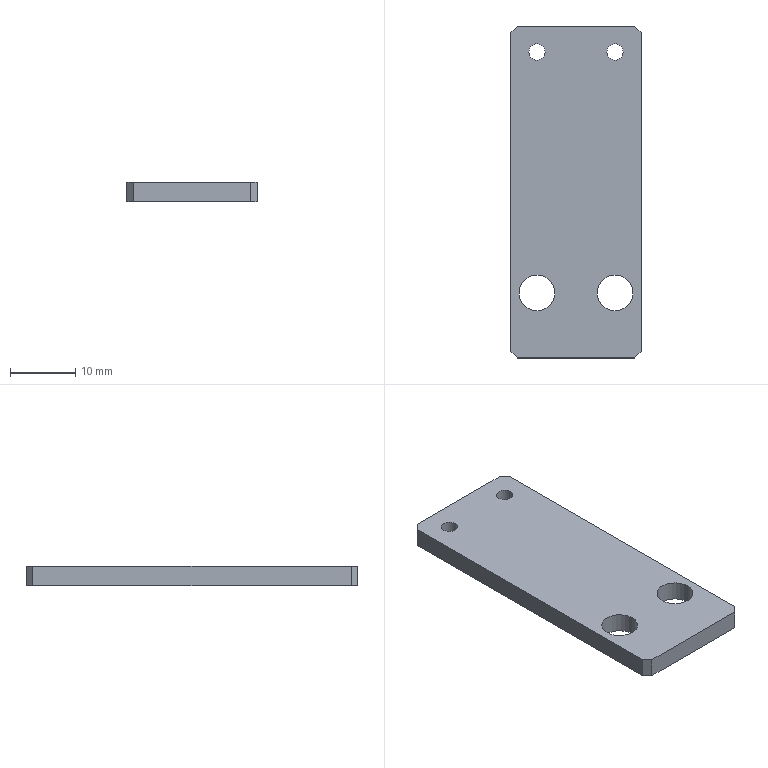Part | NX | 1 solid | 14 faces | box 20 x 51 x 3 mm | volume 2882 mm3 | plane 10 | cylinder 4 | commonest cylinder face diameters 2.5 x2 5.5 x2
STEP:
#1=CARTESIAN_POINT('',(10.,-24.5,0.));
#2=VERTEX_POINT('',#1);
#3=CARTESIAN_POINT('',(10.,24.5,0.));
#4=VERTEX_POINT('',#3);
#5=CARTESIAN_POINT('',(10.,-25.5,0.));
#6=DIRECTION('',(0.,1.,0.));
#7=VECTOR('',#6,1000.);
#8=LINE('',#5,#7);
#9=EDGE_CURVE('',#2,#4,#8,.T.);
#10=ORIENTED_EDGE('',*,*,#9,.F.);
#11=CARTESIAN_POINT('',(10.,-24.5,-3.));
#12=VERTEX_POINT('',#11);
#13=CARTESIAN_POINT('',(10.,-24.5,-3.));
#14=DIRECTION('',(0.,0.,-1.));
#15=VECTOR('',#14,1000.);
#16=LINE('',#13,#15);
#17=EDGE_CURVE('',#2,#12,#16,.T.);
#18=ORIENTED_EDGE('',*,*,#17,.T.);
#19=CARTESIAN_POINT('',(10.,24.5,-3.));
#20=VERTEX_POINT('',#19);
#21=CARTESIAN_POINT('',(10.,-25.5,-3.));
#22=DIRECTION('',(0.,1.,0.));
#23=VECTOR('',#22,1000.);
#24=LINE('',#21,#23);
#25=EDGE_CURVE('',#12,#20,#24,.T.);
#26=ORIENTED_EDGE('',*,*,#25,.T.);
#27=CARTESIAN_POINT('',(10.,24.5,-3.));
#28=DIRECTION('',(0.,0.,1.));
#29=VECTOR('',#28,1000.);
#30=LINE('',#27,#29);
#31=EDGE_CURVE('',#20,#4,#30,.T.);
#32=ORIENTED_EDGE('',*,*,#31,.T.);
#33=EDGE_LOOP('',(#10,#18,#26,#32));
#34=FACE_BOUND('',#33,.T.);
#35=CARTESIAN_POINT('',(10.,-25.5,-3.));
#36=DIRECTION('',(1.,0.,0.));
#37=DIRECTION('',(0.,0.,-1.));
#38=AXIS2_PLACEMENT_3D('',#35,#36,#37);
#39=PLANE('',#38);
#40=ADVANCED_FACE('',(#34),#39,.T.);
#41=CARTESIAN_POINT('',(-9.,-25.5,-3.));
#42=VERTEX_POINT('',#41);
#43=CARTESIAN_POINT('',(9.,-25.5,-3.));
#44=VERTEX_POINT('',#43);
#45=CARTESIAN_POINT('',(-10.,-25.5,-3.));
#46=DIRECTION('',(1.,0.,0.));
#47=VECTOR('',#46,1000.);
#48=LINE('',#45,#47);
#49=EDGE_CURVE('',#42,#44,#48,.T.);
#50=ORIENTED_EDGE('',*,*,#49,.T.);
#51=CARTESIAN_POINT('',(9.,-25.5,0.));
#52=VERTEX_POINT('',#51);
#53=CARTESIAN_POINT('',(9.,-25.5,-3.));
#54=DIRECTION('',(0.,0.,1.));
#55=VECTOR('',#54,1000.);
#56=LINE('',#53,#55);
#57=EDGE_CURVE('',#44,#52,#56,.T.);
#58=ORIENTED_EDGE('',*,*,#57,.T.);
#59=CARTESIAN_POINT('',(-9.,-25.5,0.));
#60=VERTEX_POINT('',#59);
#61=CARTESIAN_POINT('',(-10.,-25.5,0.));
#62=DIRECTION('',(1.,0.,0.));
#63=VECTOR('',#62,1000.);
#64=LINE('',#61,#63);
#65=EDGE_CURVE('',#60,#52,#64,.T.);
#66=ORIENTED_EDGE('',*,*,#65,.F.);
#67=CARTESIAN_POINT('',(-9.,-25.5,-3.));
#68=DIRECTION('',(0.,0.,-1.));
#69=VECTOR('',#68,1000.);
#70=LINE('',#67,#69);
#71=EDGE_CURVE('',#60,#42,#70,.T.);
#72=ORIENTED_EDGE('',*,*,#71,.T.);
#73=EDGE_LOOP('',(#50,#58,#66,#72));
#74=FACE_BOUND('',#73,.T.);
#75=CARTESIAN_POINT('',(-10.,-25.5,-3.));
#76=DIRECTION('',(0.,-1.,0.));
#77=DIRECTION('',(0.,0.,-1.));
#78=AXIS2_PLACEMENT_3D('',#75,#76,#77);
#79=PLANE('',#78);
#80=ADVANCED_FACE('',(#74),#79,.T.);
#81=CARTESIAN_POINT('',(-10.,24.5,-3.));
#82=VERTEX_POINT('',#81);
#83=CARTESIAN_POINT('',(-10.,-24.5,-3.));
#84=VERTEX_POINT('',#83);
#85=CARTESIAN_POINT('',(-10.,-25.5,-3.));
#86=DIRECTION('',(0.,-1.,0.));
#87=VECTOR('',#86,1000.);
#88=LINE('',#85,#87);
#89=EDGE_CURVE('',#82,#84,#88,.T.);
#90=ORIENTED_EDGE('',*,*,#89,.T.);
#91=CARTESIAN_POINT('',(-10.,-24.5,0.));
#92=VERTEX_POINT('',#91);
#93=CARTESIAN_POINT('',(-10.,-24.5,-3.));
#94=DIRECTION('',(0.,0.,1.));
#95=VECTOR('',#94,1000.);
#96=LINE('',#93,#95);
#97=EDGE_CURVE('',#84,#92,#96,.T.);
#98=ORIENTED_EDGE('',*,*,#97,.T.);
#99=CARTESIAN_POINT('',(-10.,24.5,0.));
#100=VERTEX_POINT('',#99);
#101=CARTESIAN_POINT('',(-10.,-25.5,0.));
#102=DIRECTION('',(0.,-1.,0.));
#103=VECTOR('',#102,1000.);
#104=LINE('',#101,#103);
#105=EDGE_CURVE('',#100,#92,#104,.T.);
#106=ORIENTED_EDGE('',*,*,#105,.F.);
#107=CARTESIAN_POINT('',(-10.,24.5,-3.));
#108=DIRECTION('',(0.,0.,-1.));
#109=VECTOR('',#108,1000.);
#110=LINE('',#107,#109);
#111=EDGE_CURVE('',#100,#82,#110,.T.);
#112=ORIENTED_EDGE('',*,*,#111,.T.);
#113=EDGE_LOOP('',(#90,#98,#106,#112));
#114=FACE_BOUND('',#113,.T.);
#115=CARTESIAN_POINT('',(-10.,-25.5,-3.));
#116=DIRECTION('',(-1.,0.,0.));
#117=DIRECTION('',(0.,0.,1.));
#118=AXIS2_PLACEMENT_3D('',#115,#116,#117);
#119=PLANE('',#118);
#120=ADVANCED_FACE('',(#114),#119,.T.);
#121=CARTESIAN_POINT('',(9.,25.5,0.));
#122=VERTEX_POINT('',#121);
#123=CARTESIAN_POINT('',(-9.,25.5,0.));
#124=VERTEX_POINT('',#123);
#125=CARTESIAN_POINT('',(-10.,25.5,0.));
#126=DIRECTION('',(-1.,0.,0.));
#127=VECTOR('',#126,1000.);
#128=LINE('',#125,#127);
#129=EDGE_CURVE('',#122,#124,#128,.T.);
#130=ORIENTED_EDGE('',*,*,#129,.F.);
#131=CARTESIAN_POINT('',(9.,25.5,-3.));
#132=VERTEX_POINT('',#131);
#133=CARTESIAN_POINT('',(9.,25.5,-3.));
#134=DIRECTION('',(0.,0.,-1.));
#135=VECTOR('',#134,1000.);
#136=LINE('',#133,#135);
#137=EDGE_CURVE('',#122,#132,#136,.T.);
#138=ORIENTED_EDGE('',*,*,#137,.T.);
#139=CARTESIAN_POINT('',(-9.,25.5,-3.));
#140=VERTEX_POINT('',#139);
#141=CARTESIAN_POINT('',(-10.,25.5,-3.));
#142=DIRECTION('',(-1.,0.,0.));
#143=VECTOR('',#142,1000.);
#144=LINE('',#141,#143);
#145=EDGE_CURVE('',#132,#140,#144,.T.);
#146=ORIENTED_EDGE('',*,*,#145,.T.);
#147=CARTESIAN_POINT('',(-9.,25.5,-3.));
#148=DIRECTION('',(0.,0.,1.));
#149=VECTOR('',#148,1000.);
#150=LINE('',#147,#149);
#151=EDGE_CURVE('',#140,#124,#150,.T.);
#152=ORIENTED_EDGE('',*,*,#151,.T.);
#153=EDGE_LOOP('',(#130,#138,#146,#152));
#154=FACE_BOUND('',#153,.T.);
#155=CARTESIAN_POINT('',(-10.,25.5,-3.));
#156=DIRECTION('',(0.,1.,0.));
#157=DIRECTION('',(0.,0.,1.));
#158=AXIS2_PLACEMENT_3D('',#155,#156,#157);
#159=PLANE('',#158);
#160=ADVANCED_FACE('',(#154),#159,.T.);
#161=CARTESIAN_POINT('',(-4.75,21.5,-3.));
#162=VERTEX_POINT('',#161);
#163=CARTESIAN_POINT('',(-6.,21.5,-3.));
#164=DIRECTION('',(0.,0.,1.));
#165=DIRECTION('',(1.,0.,0.));
#166=AXIS2_PLACEMENT_3D('',#163,#164,#165);
#167=CIRCLE('',#166,1.25);
#168=EDGE_CURVE('',#162,#162,#167,.T.);
#169=ORIENTED_EDGE('',*,*,#168,.T.);
#170=EDGE_LOOP('',(#169));
#171=FACE_BOUND('',#170,.T.);
#172=CARTESIAN_POINT('',(7.25,21.5,-3.));
#173=VERTEX_POINT('',#172);
#174=CARTESIAN_POINT('',(6.,21.5,-3.));
#175=DIRECTION('',(0.,0.,1.));
#176=DIRECTION('',(1.,0.,0.));
#177=AXIS2_PLACEMENT_3D('',#174,#175,#176);
#178=CIRCLE('',#177,1.25);
#179=EDGE_CURVE('',#173,#173,#178,.T.);
#180=ORIENTED_EDGE('',*,*,#179,.T.);
#181=EDGE_LOOP('',(#180));
#182=FACE_BOUND('',#181,.T.);
#183=CARTESIAN_POINT('',(-3.25,-15.5,-3.));
#184=VERTEX_POINT('',#183);
#185=CARTESIAN_POINT('',(-6.,-15.5,-3.));
#186=DIRECTION('',(0.,0.,1.));
#187=DIRECTION('',(1.,0.,0.));
#188=AXIS2_PLACEMENT_3D('',#185,#186,#187);
#189=CIRCLE('',#188,2.75);
#190=EDGE_CURVE('',#184,#184,#189,.T.);
#191=ORIENTED_EDGE('',*,*,#190,.T.);
#192=EDGE_LOOP('',(#191));
#193=FACE_BOUND('',#192,.T.);
#194=CARTESIAN_POINT('',(8.75,-15.5,-3.));
#195=VERTEX_POINT('',#194);
#196=CARTESIAN_POINT('',(6.,-15.5,-3.));
#197=DIRECTION('',(0.,0.,1.));
#198=DIRECTION('',(1.,0.,0.));
#199=AXIS2_PLACEMENT_3D('',#196,#197,#198);
#200=CIRCLE('',#199,2.75);
#201=EDGE_CURVE('',#195,#195,#200,.T.);
#202=ORIENTED_EDGE('',*,*,#201,.T.);
#203=EDGE_LOOP('',(#202));
#204=FACE_BOUND('',#203,.T.);
#205=ORIENTED_EDGE('',*,*,#25,.F.);
#206=CARTESIAN_POINT('',(17.25,-17.25,-3.));
#207=DIRECTION('',(0.7071,0.7071,0.));
#208=VECTOR('',#207,1000.);
#209=LINE('',#206,#208);
#210=EDGE_CURVE('',#12,#44,#209,.F.);
#211=ORIENTED_EDGE('',*,*,#210,.T.);
#212=ORIENTED_EDGE('',*,*,#49,.F.);
#213=CARTESIAN_POINT('',(-17.25,-17.25,-3.));
#214=DIRECTION('',(0.7071,-0.7071,0.));
#215=VECTOR('',#214,1000.);
#216=LINE('',#213,#215);
#217=EDGE_CURVE('',#42,#84,#216,.F.);
#218=ORIENTED_EDGE('',*,*,#217,.T.);
#219=ORIENTED_EDGE('',*,*,#89,.F.);
#220=CARTESIAN_POINT('',(-17.25,17.25,-3.));
#221=DIRECTION('',(-0.7071,-0.7071,0.));
#222=VECTOR('',#221,1000.);
#223=LINE('',#220,#222);
#224=EDGE_CURVE('',#82,#140,#223,.F.);
#225=ORIENTED_EDGE('',*,*,#224,.T.);
#226=ORIENTED_EDGE('',*,*,#145,.F.);
#227=CARTESIAN_POINT('',(17.25,17.25,-3.));
#228=DIRECTION('',(-0.7071,0.7071,0.));
#229=VECTOR('',#228,1000.);
#230=LINE('',#227,#229);
#231=EDGE_CURVE('',#132,#20,#230,.F.);
#232=ORIENTED_EDGE('',*,*,#231,.T.);
#233=EDGE_LOOP('',(#205,#211,#212,#218,#219,#225,#226,#232));
#234=FACE_BOUND('',#233,.T.);
#235=CARTESIAN_POINT('',(0.,0.,-3.));
#236=DIRECTION('',(0.,0.,-1.));
#237=DIRECTION('',(-1.,0.,0.));
#238=AXIS2_PLACEMENT_3D('',#235,#236,#237);
#239=PLANE('',#238);
#240=ADVANCED_FACE('',(#171,#182,#193,#204,#234),#239,.T.);
#241=CARTESIAN_POINT('',(-4.75,21.5,0.));
#242=VERTEX_POINT('',#241);
#243=CARTESIAN_POINT('',(-6.,21.5,0.));
#244=DIRECTION('',(0.,0.,1.));
#245=DIRECTION('',(1.,0.,0.));
#246=AXIS2_PLACEMENT_3D('',#243,#244,#245);
#247=CIRCLE('',#246,1.25);
#248=EDGE_CURVE('',#242,#242,#247,.T.);
#249=ORIENTED_EDGE('',*,*,#248,.F.);
#250=EDGE_LOOP('',(#249));
#251=FACE_BOUND('',#250,.T.);
#252=CARTESIAN_POINT('',(7.25,21.5,0.));
#253=VERTEX_POINT('',#252);
#254=CARTESIAN_POINT('',(6.,21.5,0.));
#255=DIRECTION('',(0.,0.,1.));
#256=DIRECTION('',(1.,0.,0.));
#257=AXIS2_PLACEMENT_3D('',#254,#255,#256);
#258=CIRCLE('',#257,1.25);
#259=EDGE_CURVE('',#253,#253,#258,.T.);
#260=ORIENTED_EDGE('',*,*,#259,.F.);
#261=EDGE_LOOP('',(#260));
#262=FACE_BOUND('',#261,.T.);
#263=CARTESIAN_POINT('',(-3.25,-15.5,0.));
#264=VERTEX_POINT('',#263);
#265=CARTESIAN_POINT('',(-6.,-15.5,0.));
#266=DIRECTION('',(0.,0.,1.));
#267=DIRECTION('',(1.,0.,0.));
#268=AXIS2_PLACEMENT_3D('',#265,#266,#267);
#269=CIRCLE('',#268,2.75);
#270=EDGE_CURVE('',#264,#264,#269,.T.);
#271=ORIENTED_EDGE('',*,*,#270,.F.);
#272=EDGE_LOOP('',(#271));
#273=FACE_BOUND('',#272,.T.);
#274=CARTESIAN_POINT('',(8.75,-15.5,0.));
#275=VERTEX_POINT('',#274);
#276=CARTESIAN_POINT('',(6.,-15.5,0.));
#277=DIRECTION('',(0.,0.,1.));
#278=DIRECTION('',(1.,0.,0.));
#279=AXIS2_PLACEMENT_3D('',#276,#277,#278);
#280=CIRCLE('',#279,2.75);
#281=EDGE_CURVE('',#275,#275,#280,.T.);
#282=ORIENTED_EDGE('',*,*,#281,.F.);
#283=EDGE_LOOP('',(#282));
#284=FACE_BOUND('',#283,.T.);
#285=ORIENTED_EDGE('',*,*,#65,.T.);
#286=CARTESIAN_POINT('',(9.,-25.5,0.));
#287=DIRECTION('',(-0.7071,-0.7071,0.));
#288=VECTOR('',#287,1000.);
#289=LINE('',#286,#288);
#290=EDGE_CURVE('',#52,#2,#289,.F.);
#291=ORIENTED_EDGE('',*,*,#290,.T.);
#292=ORIENTED_EDGE('',*,*,#9,.T.);
#293=CARTESIAN_POINT('',(10.,24.5,0.));
#294=DIRECTION('',(0.7071,-0.7071,0.));
#295=VECTOR('',#294,1000.);
#296=LINE('',#293,#295);
#297=EDGE_CURVE('',#4,#122,#296,.F.);
#298=ORIENTED_EDGE('',*,*,#297,.T.);
#299=ORIENTED_EDGE('',*,*,#129,.T.);
#300=CARTESIAN_POINT('',(-9.,25.5,0.));
#301=DIRECTION('',(0.7071,0.7071,0.));
#302=VECTOR('',#301,1000.);
#303=LINE('',#300,#302);
#304=EDGE_CURVE('',#124,#100,#303,.F.);
#305=ORIENTED_EDGE('',*,*,#304,.T.);
#306=ORIENTED_EDGE('',*,*,#105,.T.);
#307=CARTESIAN_POINT('',(-10.,-24.5,0.));
#308=DIRECTION('',(-0.7071,0.7071,0.));
#309=VECTOR('',#308,1000.);
#310=LINE('',#307,#309);
#311=EDGE_CURVE('',#92,#60,#310,.F.);
#312=ORIENTED_EDGE('',*,*,#311,.T.);
#313=EDGE_LOOP('',(#285,#291,#292,#298,#299,#305,#306,#312));
#314=FACE_BOUND('',#313,.T.);
#315=CARTESIAN_POINT('',(0.,0.,0.));
#316=DIRECTION('',(0.,0.,-1.));
#317=DIRECTION('',(-1.,0.,0.));
#318=AXIS2_PLACEMENT_3D('',#315,#316,#317);
#319=PLANE('',#318);
#320=ADVANCED_FACE('',(#251,#262,#273,#284,#314),#319,.F.);
#321=ORIENTED_EDGE('',*,*,#201,.F.);
#322=EDGE_LOOP('',(#321));
#323=FACE_BOUND('',#322,.T.);
#324=ORIENTED_EDGE('',*,*,#281,.T.);
#325=EDGE_LOOP('',(#324));
#326=FACE_BOUND('',#325,.T.);
#327=CARTESIAN_POINT('',(6.,-15.5,0.));
#328=DIRECTION('',(0.,0.,1.));
#329=DIRECTION('',(1.,0.,0.));
#330=AXIS2_PLACEMENT_3D('',#327,#328,#329);
#331=CYLINDRICAL_SURFACE('',#330,2.75);
#332=ADVANCED_FACE('',(#323,#326),#331,.F.);
#333=ORIENTED_EDGE('',*,*,#190,.F.);
#334=EDGE_LOOP('',(#333));
#335=FACE_BOUND('',#334,.T.);
#336=ORIENTED_EDGE('',*,*,#270,.T.);
#337=EDGE_LOOP('',(#336));
#338=FACE_BOUND('',#337,.T.);
#339=CARTESIAN_POINT('',(-6.,-15.5,0.));
#340=DIRECTION('',(0.,0.,1.));
#341=DIRECTION('',(1.,0.,0.));
#342=AXIS2_PLACEMENT_3D('',#339,#340,#341);
#343=CYLINDRICAL_SURFACE('',#342,2.75);
#344=ADVANCED_FACE('',(#335,#338),#343,.F.);
#345=ORIENTED_EDGE('',*,*,#210,.F.);
#346=ORIENTED_EDGE('',*,*,#17,.F.);
#347=ORIENTED_EDGE('',*,*,#290,.F.);
#348=ORIENTED_EDGE('',*,*,#57,.F.);
#349=EDGE_LOOP('',(#345,#346,#347,#348));
#350=FACE_BOUND('',#349,.T.);
#351=CARTESIAN_POINT('',(9.,-25.5,-3.));
#352=DIRECTION('',(-0.7071,0.7071,0.));
#353=DIRECTION('',(0.,0.,1.));
#354=AXIS2_PLACEMENT_3D('',#351,#352,#353);
#355=PLANE('',#354);
#356=ADVANCED_FACE('',(#350),#355,.F.);
#357=ORIENTED_EDGE('',*,*,#217,.F.);
#358=ORIENTED_EDGE('',*,*,#71,.F.);
#359=ORIENTED_EDGE('',*,*,#311,.F.);
#360=ORIENTED_EDGE('',*,*,#97,.F.);
#361=EDGE_LOOP('',(#357,#358,#359,#360));
#362=FACE_BOUND('',#361,.T.);
#363=CARTESIAN_POINT('',(-10.,-24.5,-3.));
#364=DIRECTION('',(0.7071,0.7071,0.));
#365=DIRECTION('',(0.,0.,1.));
#366=AXIS2_PLACEMENT_3D('',#363,#364,#365);
#367=PLANE('',#366);
#368=ADVANCED_FACE('',(#362),#367,.F.);
#369=ORIENTED_EDGE('',*,*,#231,.F.);
#370=ORIENTED_EDGE('',*,*,#137,.F.);
#371=ORIENTED_EDGE('',*,*,#297,.F.);
#372=ORIENTED_EDGE('',*,*,#31,.F.);
#373=EDGE_LOOP('',(#369,#370,#371,#372));
#374=FACE_BOUND('',#373,.T.);
#375=CARTESIAN_POINT('',(10.,24.5,-3.));
#376=DIRECTION('',(-0.7071,-0.7071,0.));
#377=DIRECTION('',(0.,0.,1.));
#378=AXIS2_PLACEMENT_3D('',#375,#376,#377);
#379=PLANE('',#378);
#380=ADVANCED_FACE('',(#374),#379,.F.);
#381=ORIENTED_EDGE('',*,*,#224,.F.);
#382=ORIENTED_EDGE('',*,*,#111,.F.);
#383=ORIENTED_EDGE('',*,*,#304,.F.);
#384=ORIENTED_EDGE('',*,*,#151,.F.);
#385=EDGE_LOOP('',(#381,#382,#383,#384));
#386=FACE_BOUND('',#385,.T.);
#387=CARTESIAN_POINT('',(-9.,25.5,-3.));
#388=DIRECTION('',(0.7071,-0.7071,0.));
#389=DIRECTION('',(0.,0.,1.));
#390=AXIS2_PLACEMENT_3D('',#387,#388,#389);
#391=PLANE('',#390);
#392=ADVANCED_FACE('',(#386),#391,.F.);
#393=ORIENTED_EDGE('',*,*,#179,.F.);
#394=EDGE_LOOP('',(#393));
#395=FACE_BOUND('',#394,.T.);
#396=ORIENTED_EDGE('',*,*,#259,.T.);
#397=EDGE_LOOP('',(#396));
#398=FACE_BOUND('',#397,.T.);
#399=CARTESIAN_POINT('',(6.,21.5,0.));
#400=DIRECTION('',(0.,0.,1.));
#401=DIRECTION('',(1.,0.,0.));
#402=AXIS2_PLACEMENT_3D('',#399,#400,#401);
#403=CYLINDRICAL_SURFACE('',#402,1.25);
#404=ADVANCED_FACE('',(#395,#398),#403,.F.);
#405=ORIENTED_EDGE('',*,*,#168,.F.);
#406=EDGE_LOOP('',(#405));
#407=FACE_BOUND('',#406,.T.);
#408=ORIENTED_EDGE('',*,*,#248,.T.);
#409=EDGE_LOOP('',(#408));
#410=FACE_BOUND('',#409,.T.);
#411=CARTESIAN_POINT('',(-6.,21.5,0.));
#412=DIRECTION('',(0.,0.,1.));
#413=DIRECTION('',(1.,0.,0.));
#414=AXIS2_PLACEMENT_3D('',#411,#412,#413);
#415=CYLINDRICAL_SURFACE('',#414,1.25);
#416=ADVANCED_FACE('',(#407,#410),#415,.F.);
#417=CLOSED_SHELL('',(#40,#80,#120,#160,#240,#320,#332,#344,#356,#368,#380,#392,#404,#416));
#418=MANIFOLD_SOLID_BREP('',#417);
#419=(LENGTH_UNIT()NAMED_UNIT(*)SI_UNIT(.MILLI.,.METRE.));
#420=UNCERTAINTY_MEASURE_WITH_UNIT(LENGTH_MEASURE(0.00001),#419,'','');
#421=(NAMED_UNIT(*)PLANE_ANGLE_UNIT()SI_UNIT($,.RADIAN.));
#422=(NAMED_UNIT(*)SI_UNIT($,.STERADIAN.)SOLID_ANGLE_UNIT());
#423=(GEOMETRIC_REPRESENTATION_CONTEXT(3)GLOBAL_UNCERTAINTY_ASSIGNED_CONTEXT((#420))GLOBAL_UNIT_ASSIGNED_CONTEXT((#419,#421,#422))REPRESENTATION_CONTEXT('',''));
#424=ADVANCED_BREP_SHAPE_REPRESENTATION('',(#418),#423);